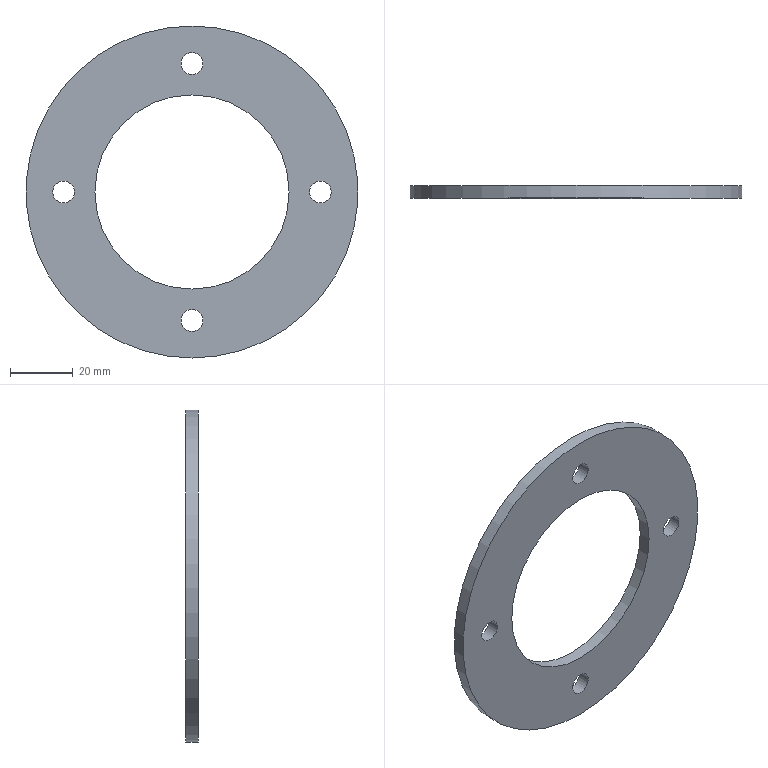Part | NX | features DATUM_CSYS 6, HOLE PACKAGE 5, SIMPLE HOLE 5, SKETCH 5, EXTRACT_DATUM_AXIS 4, EXTRACT_FACE 4, Instance Feature 3, EXTRUDE 1, OFFSET_REGION 1, Pattern Feature 1 | 1 solid | 8 faces | box 106 x 4 x 106 mm | volume 22607 mm3 | cylinder 6 | plane 2 | commonest cylinder face diameters 7 x4 62 x1 106 x1
STEP:
#1=CARTESIAN_POINT('',(0.,-4.,-53.));
#2=VERTEX_POINT('',#1);
#3=CARTESIAN_POINT('',(0.,-4.,0.));
#4=DIRECTION('',(0.,-1.,0.));
#5=DIRECTION('',(0.,0.,-1.));
#6=AXIS2_PLACEMENT_3D('',#3,#4,#5);
#7=CIRCLE('',#6,53.);
#8=EDGE_CURVE('',#2,#2,#7,.T.);
#9=ORIENTED_EDGE('',*,*,#8,.F.);
#10=EDGE_LOOP('',(#9));
#11=FACE_BOUND('',#10,.T.);
#12=CARTESIAN_POINT('',(0.,0.,-53.));
#13=VERTEX_POINT('',#12);
#14=CARTESIAN_POINT('',(0.,0.,0.));
#15=DIRECTION('',(0.,-1.,0.));
#16=DIRECTION('',(0.,0.,-1.));
#17=AXIS2_PLACEMENT_3D('',#14,#15,#16);
#18=CIRCLE('',#17,53.);
#19=EDGE_CURVE('',#13,#13,#18,.T.);
#20=ORIENTED_EDGE('',*,*,#19,.T.);
#21=EDGE_LOOP('',(#20));
#22=FACE_BOUND('',#21,.T.);
#23=CARTESIAN_POINT('',(0.,-4.,0.));
#24=DIRECTION('',(0.,1.,0.));
#25=DIRECTION('',(0.,0.,1.));
#26=AXIS2_PLACEMENT_3D('',#23,#24,#25);
#27=CYLINDRICAL_SURFACE('',#26,53.);
#28=ADVANCED_FACE('',(#11,#22),#27,.T.);
#29=CARTESIAN_POINT('',(0.,-4.,-44.5));
#30=VERTEX_POINT('',#29);
#31=CARTESIAN_POINT('',(0.,-4.,-41.));
#32=DIRECTION('',(0.,-1.,0.));
#33=DIRECTION('',(0.,0.,-1.));
#34=AXIS2_PLACEMENT_3D('',#31,#32,#33);
#35=CIRCLE('',#34,3.5);
#36=EDGE_CURVE('',#30,#30,#35,.T.);
#37=ORIENTED_EDGE('',*,*,#36,.F.);
#38=EDGE_LOOP('',(#37));
#39=FACE_BOUND('',#38,.T.);
#40=CARTESIAN_POINT('',(41.,-4.,-3.5));
#41=VERTEX_POINT('',#40);
#42=CARTESIAN_POINT('',(41.,-4.,0.));
#43=DIRECTION('',(0.,-1.,0.));
#44=DIRECTION('',(0.,0.,-1.));
#45=AXIS2_PLACEMENT_3D('',#42,#43,#44);
#46=CIRCLE('',#45,3.5);
#47=EDGE_CURVE('',#41,#41,#46,.T.);
#48=ORIENTED_EDGE('',*,*,#47,.F.);
#49=EDGE_LOOP('',(#48));
#50=FACE_BOUND('',#49,.T.);
#51=CARTESIAN_POINT('',(0.,-4.,37.5));
#52=VERTEX_POINT('',#51);
#53=CARTESIAN_POINT('',(0.,-4.,41.));
#54=DIRECTION('',(0.,-1.,0.));
#55=DIRECTION('',(0.,0.,-1.));
#56=AXIS2_PLACEMENT_3D('',#53,#54,#55);
#57=CIRCLE('',#56,3.5);
#58=EDGE_CURVE('',#52,#52,#57,.T.);
#59=ORIENTED_EDGE('',*,*,#58,.F.);
#60=EDGE_LOOP('',(#59));
#61=FACE_BOUND('',#60,.T.);
#62=CARTESIAN_POINT('',(-41.,-4.,-3.5));
#63=VERTEX_POINT('',#62);
#64=CARTESIAN_POINT('',(-41.,-4.,0.));
#65=DIRECTION('',(0.,-1.,0.));
#66=DIRECTION('',(0.,0.,-1.));
#67=AXIS2_PLACEMENT_3D('',#64,#65,#66);
#68=CIRCLE('',#67,3.5);
#69=EDGE_CURVE('',#63,#63,#68,.T.);
#70=ORIENTED_EDGE('',*,*,#69,.F.);
#71=EDGE_LOOP('',(#70));
#72=FACE_BOUND('',#71,.T.);
#73=CARTESIAN_POINT('',(0.,-4.,-31.));
#74=VERTEX_POINT('',#73);
#75=CARTESIAN_POINT('',(0.,-4.,0.));
#76=DIRECTION('',(0.,-1.,0.));
#77=DIRECTION('',(0.,0.,-1.));
#78=AXIS2_PLACEMENT_3D('',#75,#76,#77);
#79=CIRCLE('',#78,31.);
#80=EDGE_CURVE('',#74,#74,#79,.T.);
#81=ORIENTED_EDGE('',*,*,#80,.F.);
#82=EDGE_LOOP('',(#81));
#83=FACE_BOUND('',#82,.T.);
#84=ORIENTED_EDGE('',*,*,#8,.T.);
#85=EDGE_LOOP('',(#84));
#86=FACE_BOUND('',#85,.T.);
#87=CARTESIAN_POINT('',(0.,-4.,0.));
#88=DIRECTION('',(0.,-1.,0.));
#89=DIRECTION('',(0.,0.,-1.));
#90=AXIS2_PLACEMENT_3D('',#87,#88,#89);
#91=PLANE('',#90);
#92=ADVANCED_FACE('',(#39,#50,#61,#72,#83,#86),#91,.T.);
#93=CARTESIAN_POINT('',(0.,0.,-44.5));
#94=VERTEX_POINT('',#93);
#95=CARTESIAN_POINT('',(0.,0.,-41.));
#96=DIRECTION('',(0.,-1.,0.));
#97=DIRECTION('',(0.,0.,-1.));
#98=AXIS2_PLACEMENT_3D('',#95,#96,#97);
#99=CIRCLE('',#98,3.5);
#100=EDGE_CURVE('',#94,#94,#99,.T.);
#101=ORIENTED_EDGE('',*,*,#100,.T.);
#102=EDGE_LOOP('',(#101));
#103=FACE_BOUND('',#102,.T.);
#104=CARTESIAN_POINT('',(41.,0.,-3.5));
#105=VERTEX_POINT('',#104);
#106=CARTESIAN_POINT('',(41.,0.,0.));
#107=DIRECTION('',(0.,-1.,0.));
#108=DIRECTION('',(0.,0.,-1.));
#109=AXIS2_PLACEMENT_3D('',#106,#107,#108);
#110=CIRCLE('',#109,3.5);
#111=EDGE_CURVE('',#105,#105,#110,.T.);
#112=ORIENTED_EDGE('',*,*,#111,.T.);
#113=EDGE_LOOP('',(#112));
#114=FACE_BOUND('',#113,.T.);
#115=CARTESIAN_POINT('',(0.,0.,37.5));
#116=VERTEX_POINT('',#115);
#117=CARTESIAN_POINT('',(0.,0.,41.));
#118=DIRECTION('',(0.,-1.,0.));
#119=DIRECTION('',(0.,0.,-1.));
#120=AXIS2_PLACEMENT_3D('',#117,#118,#119);
#121=CIRCLE('',#120,3.5);
#122=EDGE_CURVE('',#116,#116,#121,.T.);
#123=ORIENTED_EDGE('',*,*,#122,.T.);
#124=EDGE_LOOP('',(#123));
#125=FACE_BOUND('',#124,.T.);
#126=CARTESIAN_POINT('',(-41.,0.,-3.5));
#127=VERTEX_POINT('',#126);
#128=CARTESIAN_POINT('',(-41.,0.,0.));
#129=DIRECTION('',(0.,-1.,0.));
#130=DIRECTION('',(0.,0.,-1.));
#131=AXIS2_PLACEMENT_3D('',#128,#129,#130);
#132=CIRCLE('',#131,3.5);
#133=EDGE_CURVE('',#127,#127,#132,.T.);
#134=ORIENTED_EDGE('',*,*,#133,.T.);
#135=EDGE_LOOP('',(#134));
#136=FACE_BOUND('',#135,.T.);
#137=CARTESIAN_POINT('',(0.,0.,-31.));
#138=VERTEX_POINT('',#137);
#139=CARTESIAN_POINT('',(0.,0.,0.));
#140=DIRECTION('',(0.,-1.,0.));
#141=DIRECTION('',(0.,0.,-1.));
#142=AXIS2_PLACEMENT_3D('',#139,#140,#141);
#143=CIRCLE('',#142,31.);
#144=EDGE_CURVE('',#138,#138,#143,.T.);
#145=ORIENTED_EDGE('',*,*,#144,.T.);
#146=EDGE_LOOP('',(#145));
#147=FACE_BOUND('',#146,.T.);
#148=ORIENTED_EDGE('',*,*,#19,.F.);
#149=EDGE_LOOP('',(#148));
#150=FACE_BOUND('',#149,.T.);
#151=CARTESIAN_POINT('',(0.,0.,0.));
#152=DIRECTION('',(0.,-1.,0.));
#153=DIRECTION('',(0.,0.,-1.));
#154=AXIS2_PLACEMENT_3D('',#151,#152,#153);
#155=PLANE('',#154);
#156=ADVANCED_FACE('',(#103,#114,#125,#136,#147,#150),#155,.F.);
#157=ORIENTED_EDGE('',*,*,#80,.T.);
#158=EDGE_LOOP('',(#157));
#159=FACE_BOUND('',#158,.T.);
#160=ORIENTED_EDGE('',*,*,#144,.F.);
#161=EDGE_LOOP('',(#160));
#162=FACE_BOUND('',#161,.T.);
#163=CARTESIAN_POINT('',(0.,0.,0.));
#164=DIRECTION('',(0.,-1.,0.));
#165=DIRECTION('',(0.,0.,-1.));
#166=AXIS2_PLACEMENT_3D('',#163,#164,#165);
#167=CYLINDRICAL_SURFACE('',#166,31.);
#168=ADVANCED_FACE('',(#159,#162),#167,.F.);
#169=ORIENTED_EDGE('',*,*,#69,.T.);
#170=EDGE_LOOP('',(#169));
#171=FACE_BOUND('',#170,.T.);
#172=ORIENTED_EDGE('',*,*,#133,.F.);
#173=EDGE_LOOP('',(#172));
#174=FACE_BOUND('',#173,.T.);
#175=CARTESIAN_POINT('',(-41.,0.,0.));
#176=DIRECTION('',(0.,-1.,0.));
#177=DIRECTION('',(0.,0.,-1.));
#178=AXIS2_PLACEMENT_3D('',#175,#176,#177);
#179=CYLINDRICAL_SURFACE('',#178,3.5);
#180=ADVANCED_FACE('',(#171,#174),#179,.F.);
#181=ORIENTED_EDGE('',*,*,#58,.T.);
#182=EDGE_LOOP('',(#181));
#183=FACE_BOUND('',#182,.T.);
#184=ORIENTED_EDGE('',*,*,#122,.F.);
#185=EDGE_LOOP('',(#184));
#186=FACE_BOUND('',#185,.T.);
#187=CARTESIAN_POINT('',(0.,0.,41.));
#188=DIRECTION('',(0.,-1.,0.));
#189=DIRECTION('',(0.,0.,-1.));
#190=AXIS2_PLACEMENT_3D('',#187,#188,#189);
#191=CYLINDRICAL_SURFACE('',#190,3.5);
#192=ADVANCED_FACE('',(#183,#186),#191,.F.);
#193=ORIENTED_EDGE('',*,*,#47,.T.);
#194=EDGE_LOOP('',(#193));
#195=FACE_BOUND('',#194,.T.);
#196=ORIENTED_EDGE('',*,*,#111,.F.);
#197=EDGE_LOOP('',(#196));
#198=FACE_BOUND('',#197,.T.);
#199=CARTESIAN_POINT('',(41.,0.,0.));
#200=DIRECTION('',(0.,-1.,0.));
#201=DIRECTION('',(0.,0.,-1.));
#202=AXIS2_PLACEMENT_3D('',#199,#200,#201);
#203=CYLINDRICAL_SURFACE('',#202,3.5);
#204=ADVANCED_FACE('',(#195,#198),#203,.F.);
#205=ORIENTED_EDGE('',*,*,#36,.T.);
#206=EDGE_LOOP('',(#205));
#207=FACE_BOUND('',#206,.T.);
#208=ORIENTED_EDGE('',*,*,#100,.F.);
#209=EDGE_LOOP('',(#208));
#210=FACE_BOUND('',#209,.T.);
#211=CARTESIAN_POINT('',(0.,0.,-41.));
#212=DIRECTION('',(0.,-1.,0.));
#213=DIRECTION('',(0.,0.,-1.));
#214=AXIS2_PLACEMENT_3D('',#211,#212,#213);
#215=CYLINDRICAL_SURFACE('',#214,3.5);
#216=ADVANCED_FACE('',(#207,#210),#215,.F.);
#217=CLOSED_SHELL('',(#28,#92,#156,#168,#180,#192,#204,#216));
#218=MANIFOLD_SOLID_BREP('',#217);
#219=(LENGTH_UNIT()NAMED_UNIT(*)SI_UNIT(.MILLI.,.METRE.));
#220=UNCERTAINTY_MEASURE_WITH_UNIT(LENGTH_MEASURE(0.00001),#219,'','');
#221=(NAMED_UNIT(*)PLANE_ANGLE_UNIT()SI_UNIT($,.RADIAN.));
#222=(NAMED_UNIT(*)SI_UNIT($,.STERADIAN.)SOLID_ANGLE_UNIT());
#223=(GEOMETRIC_REPRESENTATION_CONTEXT(3)GLOBAL_UNCERTAINTY_ASSIGNED_CONTEXT((#220))GLOBAL_UNIT_ASSIGNED_CONTEXT((#219,#221,#222))REPRESENTATION_CONTEXT('',''));
#224=ADVANCED_BREP_SHAPE_REPRESENTATION('',(#218),#223);